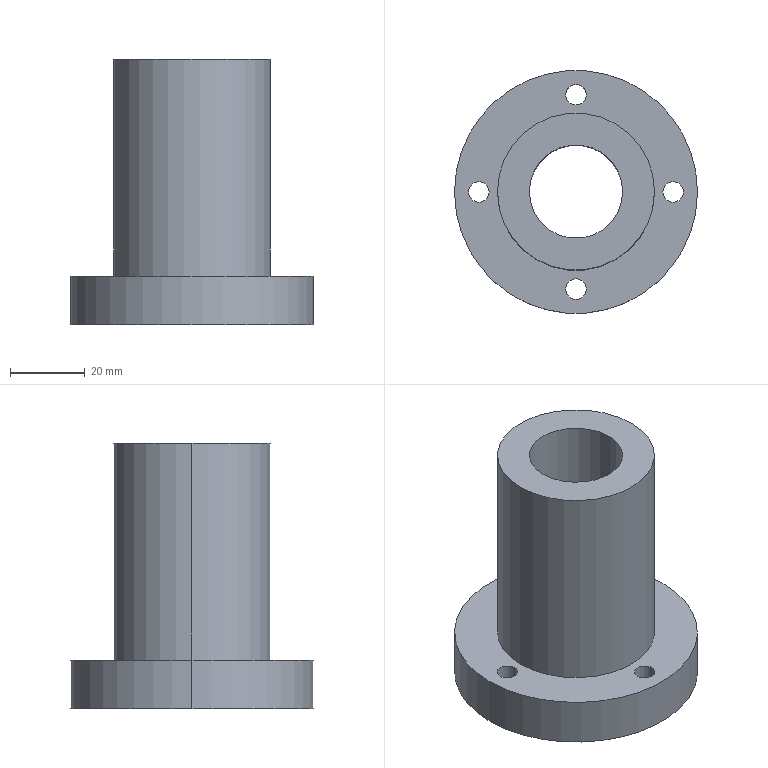Part | SolidWorks | features 3DProfileFeature 1, Extrusion 1, HoleWzd 1, ICE 1 | 1 solid | 29 faces | box 65 x 65 x 71 mm | volume 86157 mm3 | cylinder 22 | plane 7 | commonest cylinder face diameters 5.5 x8 10 x8 25 x2 42 x2 65 x2
STEP:
#1=CARTESIAN_POINT('',(5.,26.,5.7));
#2=VERTEX_POINT('',#1);
#3=CARTESIAN_POINT('',(-5.,26.,5.7));
#4=VERTEX_POINT('',#3);
#5=CARTESIAN_POINT('',(0.,26.,5.7));
#6=DIRECTION('',(0.,0.,-1.));
#7=DIRECTION('',(-1.,0.,0.));
#8=AXIS2_PLACEMENT_3D('',#5,#6,#7);
#9=CIRCLE('',#8,5.);
#10=EDGE_CURVE('',#2,#4,#9,.T.);
#11=ORIENTED_EDGE('',*,*,#10,.F.);
#12=CARTESIAN_POINT('',(5.,26.,0.));
#13=VERTEX_POINT('',#12);
#14=CARTESIAN_POINT('',(5.,26.,0.));
#15=DIRECTION('',(0.,0.,-1.));
#16=VECTOR('',#15,1000.);
#17=LINE('',#14,#16);
#18=EDGE_CURVE('',#2,#13,#17,.T.);
#19=ORIENTED_EDGE('',*,*,#18,.T.);
#20=CARTESIAN_POINT('',(-5.,26.,0.));
#21=VERTEX_POINT('',#20);
#22=CARTESIAN_POINT('',(0.,26.,0.));
#23=DIRECTION('',(0.,0.,-1.));
#24=DIRECTION('',(-1.,0.,0.));
#25=AXIS2_PLACEMENT_3D('',#22,#23,#24);
#26=CIRCLE('',#25,5.);
#27=EDGE_CURVE('',#13,#21,#26,.T.);
#28=ORIENTED_EDGE('',*,*,#27,.T.);
#29=CARTESIAN_POINT('',(-5.,26.,0.));
#30=DIRECTION('',(0.,0.,-1.));
#31=VECTOR('',#30,1000.);
#32=LINE('',#29,#31);
#33=EDGE_CURVE('',#4,#21,#32,.T.);
#34=ORIENTED_EDGE('',*,*,#33,.F.);
#35=EDGE_LOOP('',(#11,#19,#28,#34));
#36=FACE_OUTER_BOUND('',#35,.T.);
#37=CARTESIAN_POINT('',(0.,26.,0.));
#38=DIRECTION('',(0.,0.,-1.));
#39=DIRECTION('',(-1.,0.,0.));
#40=AXIS2_PLACEMENT_3D('',#37,#38,#39);
#41=CYLINDRICAL_SURFACE('',#40,5.);
#42=ADVANCED_FACE('',(#36),#41,.F.);
#43=CARTESIAN_POINT('',(2.75,26.,13.));
#44=VERTEX_POINT('',#43);
#45=CARTESIAN_POINT('',(-2.75,26.,13.));
#46=VERTEX_POINT('',#45);
#47=CARTESIAN_POINT('',(0.,26.,13.));
#48=DIRECTION('',(0.,0.,-1.));
#49=DIRECTION('',(-1.,0.,0.));
#50=AXIS2_PLACEMENT_3D('',#47,#48,#49);
#51=CIRCLE('',#50,2.75);
#52=EDGE_CURVE('',#44,#46,#51,.T.);
#53=ORIENTED_EDGE('',*,*,#52,.F.);
#54=CARTESIAN_POINT('',(2.75,26.,5.7));
#55=VERTEX_POINT('',#54);
#56=CARTESIAN_POINT('',(2.75,26.,0.));
#57=DIRECTION('',(0.,0.,-1.));
#58=VECTOR('',#57,1000.);
#59=LINE('',#56,#58);
#60=EDGE_CURVE('',#44,#55,#59,.T.);
#61=ORIENTED_EDGE('',*,*,#60,.T.);
#62=CARTESIAN_POINT('',(-2.75,26.,5.7));
#63=VERTEX_POINT('',#62);
#64=CARTESIAN_POINT('',(0.,26.,5.7));
#65=DIRECTION('',(0.,0.,-1.));
#66=DIRECTION('',(-1.,0.,0.));
#67=AXIS2_PLACEMENT_3D('',#64,#65,#66);
#68=CIRCLE('',#67,2.75);
#69=EDGE_CURVE('',#55,#63,#68,.T.);
#70=ORIENTED_EDGE('',*,*,#69,.T.);
#71=CARTESIAN_POINT('',(-2.75,26.,0.));
#72=DIRECTION('',(0.,0.,-1.));
#73=VECTOR('',#72,1000.);
#74=LINE('',#71,#73);
#75=EDGE_CURVE('',#46,#63,#74,.T.);
#76=ORIENTED_EDGE('',*,*,#75,.F.);
#77=EDGE_LOOP('',(#53,#61,#70,#76));
#78=FACE_OUTER_BOUND('',#77,.T.);
#79=CARTESIAN_POINT('',(0.,26.,0.));
#80=DIRECTION('',(0.,0.,-1.));
#81=DIRECTION('',(-1.,0.,0.));
#82=AXIS2_PLACEMENT_3D('',#79,#80,#81);
#83=CYLINDRICAL_SURFACE('',#82,2.75);
#84=ADVANCED_FACE('',(#78),#83,.F.);
#85=CARTESIAN_POINT('',(-21.,0.,5.7));
#86=VERTEX_POINT('',#85);
#87=CARTESIAN_POINT('',(-31.,0.,5.7));
#88=VERTEX_POINT('',#87);
#89=CARTESIAN_POINT('',(-26.,0.,5.7));
#90=DIRECTION('',(0.,0.,-1.));
#91=DIRECTION('',(-1.,0.,0.));
#92=AXIS2_PLACEMENT_3D('',#89,#90,#91);
#93=CIRCLE('',#92,5.);
#94=EDGE_CURVE('',#86,#88,#93,.T.);
#95=ORIENTED_EDGE('',*,*,#94,.F.);
#96=CARTESIAN_POINT('',(-21.,0.,0.));
#97=VERTEX_POINT('',#96);
#98=CARTESIAN_POINT('',(-21.,0.,0.));
#99=DIRECTION('',(0.,0.,-1.));
#100=VECTOR('',#99,1000.);
#101=LINE('',#98,#100);
#102=EDGE_CURVE('',#86,#97,#101,.T.);
#103=ORIENTED_EDGE('',*,*,#102,.T.);
#104=CARTESIAN_POINT('',(-31.,0.,0.));
#105=VERTEX_POINT('',#104);
#106=CARTESIAN_POINT('',(-26.,0.,0.));
#107=DIRECTION('',(0.,0.,-1.));
#108=DIRECTION('',(-1.,0.,0.));
#109=AXIS2_PLACEMENT_3D('',#106,#107,#108);
#110=CIRCLE('',#109,5.);
#111=EDGE_CURVE('',#97,#105,#110,.T.);
#112=ORIENTED_EDGE('',*,*,#111,.T.);
#113=CARTESIAN_POINT('',(-31.,0.,0.));
#114=DIRECTION('',(0.,0.,-1.));
#115=VECTOR('',#114,1000.);
#116=LINE('',#113,#115);
#117=EDGE_CURVE('',#88,#105,#116,.T.);
#118=ORIENTED_EDGE('',*,*,#117,.F.);
#119=EDGE_LOOP('',(#95,#103,#112,#118));
#120=FACE_OUTER_BOUND('',#119,.T.);
#121=CARTESIAN_POINT('',(-26.,0.,0.));
#122=DIRECTION('',(0.,0.,-1.));
#123=DIRECTION('',(-1.,0.,0.));
#124=AXIS2_PLACEMENT_3D('',#121,#122,#123);
#125=CYLINDRICAL_SURFACE('',#124,5.);
#126=ADVANCED_FACE('',(#120),#125,.F.);
#127=CARTESIAN_POINT('',(-23.25,0.,13.));
#128=VERTEX_POINT('',#127);
#129=CARTESIAN_POINT('',(-28.75,0.,13.));
#130=VERTEX_POINT('',#129);
#131=CARTESIAN_POINT('',(-26.,0.,13.));
#132=DIRECTION('',(0.,0.,-1.));
#133=DIRECTION('',(-1.,0.,0.));
#134=AXIS2_PLACEMENT_3D('',#131,#132,#133);
#135=CIRCLE('',#134,2.75);
#136=EDGE_CURVE('',#128,#130,#135,.T.);
#137=ORIENTED_EDGE('',*,*,#136,.F.);
#138=CARTESIAN_POINT('',(-23.25,0.,5.7));
#139=VERTEX_POINT('',#138);
#140=CARTESIAN_POINT('',(-23.25,0.,0.));
#141=DIRECTION('',(0.,0.,-1.));
#142=VECTOR('',#141,1000.);
#143=LINE('',#140,#142);
#144=EDGE_CURVE('',#128,#139,#143,.T.);
#145=ORIENTED_EDGE('',*,*,#144,.T.);
#146=CARTESIAN_POINT('',(-28.75,0.,5.7));
#147=VERTEX_POINT('',#146);
#148=CARTESIAN_POINT('',(-26.,0.,5.7));
#149=DIRECTION('',(0.,0.,-1.));
#150=DIRECTION('',(-1.,0.,0.));
#151=AXIS2_PLACEMENT_3D('',#148,#149,#150);
#152=CIRCLE('',#151,2.75);
#153=EDGE_CURVE('',#139,#147,#152,.T.);
#154=ORIENTED_EDGE('',*,*,#153,.T.);
#155=CARTESIAN_POINT('',(-28.75,0.,0.));
#156=DIRECTION('',(0.,0.,-1.));
#157=VECTOR('',#156,1000.);
#158=LINE('',#155,#157);
#159=EDGE_CURVE('',#130,#147,#158,.T.);
#160=ORIENTED_EDGE('',*,*,#159,.F.);
#161=EDGE_LOOP('',(#137,#145,#154,#160));
#162=FACE_OUTER_BOUND('',#161,.T.);
#163=CARTESIAN_POINT('',(-26.,0.,0.));
#164=DIRECTION('',(0.,0.,-1.));
#165=DIRECTION('',(-1.,0.,0.));
#166=AXIS2_PLACEMENT_3D('',#163,#164,#165);
#167=CYLINDRICAL_SURFACE('',#166,2.75);
#168=ADVANCED_FACE('',(#162),#167,.F.);
#169=CARTESIAN_POINT('',(5.,-26.,5.7));
#170=VERTEX_POINT('',#169);
#171=CARTESIAN_POINT('',(-5.,-26.,5.7));
#172=VERTEX_POINT('',#171);
#173=CARTESIAN_POINT('',(0.,-26.,5.7));
#174=DIRECTION('',(0.,0.,-1.));
#175=DIRECTION('',(-1.,0.,0.));
#176=AXIS2_PLACEMENT_3D('',#173,#174,#175);
#177=CIRCLE('',#176,5.);
#178=EDGE_CURVE('',#170,#172,#177,.T.);
#179=ORIENTED_EDGE('',*,*,#178,.F.);
#180=CARTESIAN_POINT('',(5.,-26.,0.));
#181=VERTEX_POINT('',#180);
#182=CARTESIAN_POINT('',(5.,-26.,0.));
#183=DIRECTION('',(0.,0.,-1.));
#184=VECTOR('',#183,1000.);
#185=LINE('',#182,#184);
#186=EDGE_CURVE('',#170,#181,#185,.T.);
#187=ORIENTED_EDGE('',*,*,#186,.T.);
#188=CARTESIAN_POINT('',(-5.,-26.,0.));
#189=VERTEX_POINT('',#188);
#190=CARTESIAN_POINT('',(0.,-26.,0.));
#191=DIRECTION('',(0.,0.,-1.));
#192=DIRECTION('',(-1.,0.,0.));
#193=AXIS2_PLACEMENT_3D('',#190,#191,#192);
#194=CIRCLE('',#193,5.);
#195=EDGE_CURVE('',#181,#189,#194,.T.);
#196=ORIENTED_EDGE('',*,*,#195,.T.);
#197=CARTESIAN_POINT('',(-5.,-26.,0.));
#198=DIRECTION('',(0.,0.,-1.));
#199=VECTOR('',#198,1000.);
#200=LINE('',#197,#199);
#201=EDGE_CURVE('',#172,#189,#200,.T.);
#202=ORIENTED_EDGE('',*,*,#201,.F.);
#203=EDGE_LOOP('',(#179,#187,#196,#202));
#204=FACE_OUTER_BOUND('',#203,.T.);
#205=CARTESIAN_POINT('',(0.,-26.,0.));
#206=DIRECTION('',(0.,0.,-1.));
#207=DIRECTION('',(-1.,0.,0.));
#208=AXIS2_PLACEMENT_3D('',#205,#206,#207);
#209=CYLINDRICAL_SURFACE('',#208,5.);
#210=ADVANCED_FACE('',(#204),#209,.F.);
#211=CARTESIAN_POINT('',(2.75,-26.,13.));
#212=VERTEX_POINT('',#211);
#213=CARTESIAN_POINT('',(-2.75,-26.,13.));
#214=VERTEX_POINT('',#213);
#215=CARTESIAN_POINT('',(0.,-26.,13.));
#216=DIRECTION('',(0.,0.,-1.));
#217=DIRECTION('',(-1.,0.,0.));
#218=AXIS2_PLACEMENT_3D('',#215,#216,#217);
#219=CIRCLE('',#218,2.75);
#220=EDGE_CURVE('',#212,#214,#219,.T.);
#221=ORIENTED_EDGE('',*,*,#220,.F.);
#222=CARTESIAN_POINT('',(2.75,-26.,5.7));
#223=VERTEX_POINT('',#222);
#224=CARTESIAN_POINT('',(2.75,-26.,0.));
#225=DIRECTION('',(0.,0.,-1.));
#226=VECTOR('',#225,1000.);
#227=LINE('',#224,#226);
#228=EDGE_CURVE('',#212,#223,#227,.T.);
#229=ORIENTED_EDGE('',*,*,#228,.T.);
#230=CARTESIAN_POINT('',(-2.75,-26.,5.7));
#231=VERTEX_POINT('',#230);
#232=CARTESIAN_POINT('',(0.,-26.,5.7));
#233=DIRECTION('',(0.,0.,-1.));
#234=DIRECTION('',(-1.,0.,0.));
#235=AXIS2_PLACEMENT_3D('',#232,#233,#234);
#236=CIRCLE('',#235,2.75);
#237=EDGE_CURVE('',#223,#231,#236,.T.);
#238=ORIENTED_EDGE('',*,*,#237,.T.);
#239=CARTESIAN_POINT('',(-2.75,-26.,0.));
#240=DIRECTION('',(0.,0.,-1.));
#241=VECTOR('',#240,1000.);
#242=LINE('',#239,#241);
#243=EDGE_CURVE('',#214,#231,#242,.T.);
#244=ORIENTED_EDGE('',*,*,#243,.F.);
#245=EDGE_LOOP('',(#221,#229,#238,#244));
#246=FACE_OUTER_BOUND('',#245,.T.);
#247=CARTESIAN_POINT('',(0.,-26.,0.));
#248=DIRECTION('',(0.,0.,-1.));
#249=DIRECTION('',(-1.,0.,0.));
#250=AXIS2_PLACEMENT_3D('',#247,#248,#249);
#251=CYLINDRICAL_SURFACE('',#250,2.75);
#252=ADVANCED_FACE('',(#246),#251,.F.);
#253=CARTESIAN_POINT('',(31.,0.,5.7));
#254=VERTEX_POINT('',#253);
#255=CARTESIAN_POINT('',(21.,0.,5.7));
#256=VERTEX_POINT('',#255);
#257=CARTESIAN_POINT('',(26.,0.,5.7));
#258=DIRECTION('',(0.,0.,-1.));
#259=DIRECTION('',(-1.,0.,0.));
#260=AXIS2_PLACEMENT_3D('',#257,#258,#259);
#261=CIRCLE('',#260,5.);
#262=EDGE_CURVE('',#254,#256,#261,.T.);
#263=ORIENTED_EDGE('',*,*,#262,.F.);
#264=CARTESIAN_POINT('',(31.,0.,0.));
#265=VERTEX_POINT('',#264);
#266=CARTESIAN_POINT('',(31.,0.,0.));
#267=DIRECTION('',(0.,0.,-1.));
#268=VECTOR('',#267,1000.);
#269=LINE('',#266,#268);
#270=EDGE_CURVE('',#254,#265,#269,.T.);
#271=ORIENTED_EDGE('',*,*,#270,.T.);
#272=CARTESIAN_POINT('',(21.,0.,0.));
#273=VERTEX_POINT('',#272);
#274=CARTESIAN_POINT('',(26.,0.,0.));
#275=DIRECTION('',(0.,0.,-1.));
#276=DIRECTION('',(-1.,0.,0.));
#277=AXIS2_PLACEMENT_3D('',#274,#275,#276);
#278=CIRCLE('',#277,5.);
#279=EDGE_CURVE('',#265,#273,#278,.T.);
#280=ORIENTED_EDGE('',*,*,#279,.T.);
#281=CARTESIAN_POINT('',(21.,0.,0.));
#282=DIRECTION('',(0.,0.,-1.));
#283=VECTOR('',#282,1000.);
#284=LINE('',#281,#283);
#285=EDGE_CURVE('',#256,#273,#284,.T.);
#286=ORIENTED_EDGE('',*,*,#285,.F.);
#287=EDGE_LOOP('',(#263,#271,#280,#286));
#288=FACE_OUTER_BOUND('',#287,.T.);
#289=CARTESIAN_POINT('',(26.,0.,0.));
#290=DIRECTION('',(0.,0.,-1.));
#291=DIRECTION('',(-1.,0.,0.));
#292=AXIS2_PLACEMENT_3D('',#289,#290,#291);
#293=CYLINDRICAL_SURFACE('',#292,5.);
#294=ADVANCED_FACE('',(#288),#293,.F.);
#295=CARTESIAN_POINT('',(28.75,0.,13.));
#296=VERTEX_POINT('',#295);
#297=CARTESIAN_POINT('',(23.25,0.,13.));
#298=VERTEX_POINT('',#297);
#299=CARTESIAN_POINT('',(26.,0.,13.));
#300=DIRECTION('',(0.,0.,-1.));
#301=DIRECTION('',(-1.,0.,0.));
#302=AXIS2_PLACEMENT_3D('',#299,#300,#301);
#303=CIRCLE('',#302,2.75);
#304=EDGE_CURVE('',#296,#298,#303,.T.);
#305=ORIENTED_EDGE('',*,*,#304,.F.);
#306=CARTESIAN_POINT('',(28.75,0.,5.7));
#307=VERTEX_POINT('',#306);
#308=CARTESIAN_POINT('',(28.75,0.,0.));
#309=DIRECTION('',(0.,0.,-1.));
#310=VECTOR('',#309,1000.);
#311=LINE('',#308,#310);
#312=EDGE_CURVE('',#296,#307,#311,.T.);
#313=ORIENTED_EDGE('',*,*,#312,.T.);
#314=CARTESIAN_POINT('',(23.25,0.,5.7));
#315=VERTEX_POINT('',#314);
#316=CARTESIAN_POINT('',(26.,0.,5.7));
#317=DIRECTION('',(0.,0.,-1.));
#318=DIRECTION('',(-1.,0.,0.));
#319=AXIS2_PLACEMENT_3D('',#316,#317,#318);
#320=CIRCLE('',#319,2.75);
#321=EDGE_CURVE('',#307,#315,#320,.T.);
#322=ORIENTED_EDGE('',*,*,#321,.T.);
#323=CARTESIAN_POINT('',(23.25,0.,0.));
#324=DIRECTION('',(0.,0.,-1.));
#325=VECTOR('',#324,1000.);
#326=LINE('',#323,#325);
#327=EDGE_CURVE('',#298,#315,#326,.T.);
#328=ORIENTED_EDGE('',*,*,#327,.F.);
#329=EDGE_LOOP('',(#305,#313,#322,#328));
#330=FACE_OUTER_BOUND('',#329,.T.);
#331=CARTESIAN_POINT('',(26.,0.,0.));
#332=DIRECTION('',(0.,0.,-1.));
#333=DIRECTION('',(-1.,0.,0.));
#334=AXIS2_PLACEMENT_3D('',#331,#332,#333);
#335=CYLINDRICAL_SURFACE('',#334,2.75);
#336=ADVANCED_FACE('',(#330),#335,.F.);
#337=CARTESIAN_POINT('',(-32.5,0.,13.));
#338=VERTEX_POINT('',#337);
#339=CARTESIAN_POINT('',(32.5,0.,13.));
#340=VERTEX_POINT('',#339);
#341=CARTESIAN_POINT('',(0.,0.,13.));
#342=DIRECTION('',(0.,0.,-1.));
#343=DIRECTION('',(-1.,0.,0.));
#344=AXIS2_PLACEMENT_3D('',#341,#342,#343);
#345=CIRCLE('',#344,32.5);
#346=EDGE_CURVE('',#338,#340,#345,.T.);
#347=ORIENTED_EDGE('',*,*,#346,.T.);
#348=CARTESIAN_POINT('',(32.5,0.,0.));
#349=VERTEX_POINT('',#348);
#350=CARTESIAN_POINT('',(32.5,0.,13.));
#351=DIRECTION('',(0.,0.,-1.));
#352=VECTOR('',#351,1000.);
#353=LINE('',#350,#352);
#354=EDGE_CURVE('',#340,#349,#353,.T.);
#355=ORIENTED_EDGE('',*,*,#354,.T.);
#356=CARTESIAN_POINT('',(-32.5,0.,0.));
#357=VERTEX_POINT('',#356);
#358=CARTESIAN_POINT('',(0.,0.,0.));
#359=DIRECTION('',(0.,0.,-1.));
#360=DIRECTION('',(-1.,0.,0.));
#361=AXIS2_PLACEMENT_3D('',#358,#359,#360);
#362=CIRCLE('',#361,32.5);
#363=EDGE_CURVE('',#357,#349,#362,.T.);
#364=ORIENTED_EDGE('',*,*,#363,.F.);
#365=CARTESIAN_POINT('',(-32.5,0.,13.));
#366=DIRECTION('',(0.,0.,-1.));
#367=VECTOR('',#366,1000.);
#368=LINE('',#365,#367);
#369=EDGE_CURVE('',#338,#357,#368,.T.);
#370=ORIENTED_EDGE('',*,*,#369,.F.);
#371=EDGE_LOOP('',(#347,#355,#364,#370));
#372=FACE_OUTER_BOUND('',#371,.T.);
#373=CARTESIAN_POINT('',(0.,0.,13.));
#374=DIRECTION('',(0.,0.,-1.));
#375=DIRECTION('',(-1.,0.,0.));
#376=AXIS2_PLACEMENT_3D('',#373,#374,#375);
#377=CYLINDRICAL_SURFACE('',#376,32.5);
#378=ADVANCED_FACE('',(#372),#377,.T.);
#379=CARTESIAN_POINT('',(-12.5,0.,71.));
#380=VERTEX_POINT('',#379);
#381=CARTESIAN_POINT('',(12.5,0.,71.));
#382=VERTEX_POINT('',#381);
#383=CARTESIAN_POINT('',(0.,0.,71.));
#384=DIRECTION('',(0.,0.,1.));
#385=DIRECTION('',(1.,0.,0.));
#386=AXIS2_PLACEMENT_3D('',#383,#384,#385);
#387=CIRCLE('',#386,12.5);
#388=EDGE_CURVE('',#380,#382,#387,.T.);
#389=ORIENTED_EDGE('',*,*,#388,.T.);
#390=CARTESIAN_POINT('',(12.5,0.,0.));
#391=VERTEX_POINT('',#390);
#392=CARTESIAN_POINT('',(12.5,0.,71.));
#393=DIRECTION('',(0.,0.,-1.));
#394=VECTOR('',#393,1000.);
#395=LINE('',#392,#394);
#396=EDGE_CURVE('',#382,#391,#395,.T.);
#397=ORIENTED_EDGE('',*,*,#396,.T.);
#398=CARTESIAN_POINT('',(-12.5,0.,0.));
#399=VERTEX_POINT('',#398);
#400=CARTESIAN_POINT('',(0.,0.,0.));
#401=DIRECTION('',(0.,0.,1.));
#402=DIRECTION('',(1.,0.,0.));
#403=AXIS2_PLACEMENT_3D('',#400,#401,#402);
#404=CIRCLE('',#403,12.5);
#405=EDGE_CURVE('',#399,#391,#404,.T.);
#406=ORIENTED_EDGE('',*,*,#405,.F.);
#407=CARTESIAN_POINT('',(-12.5,0.,71.));
#408=DIRECTION('',(0.,0.,-1.));
#409=VECTOR('',#408,1000.);
#410=LINE('',#407,#409);
#411=EDGE_CURVE('',#380,#399,#410,.T.);
#412=ORIENTED_EDGE('',*,*,#411,.F.);
#413=EDGE_LOOP('',(#389,#397,#406,#412));
#414=FACE_OUTER_BOUND('',#413,.T.);
#415=CARTESIAN_POINT('',(0.,0.,71.));
#416=DIRECTION('',(0.,0.,-1.));
#417=DIRECTION('',(-1.,0.,0.));
#418=AXIS2_PLACEMENT_3D('',#415,#416,#417);
#419=CYLINDRICAL_SURFACE('',#418,12.5);
#420=ADVANCED_FACE('',(#414),#419,.F.);
#421=CARTESIAN_POINT('',(21.,0.,71.));
#422=VERTEX_POINT('',#421);
#423=CARTESIAN_POINT('',(-21.,0.,71.));
#424=VERTEX_POINT('',#423);
#425=CARTESIAN_POINT('',(0.,0.,71.));
#426=DIRECTION('',(0.,0.,1.));
#427=DIRECTION('',(1.,0.,0.));
#428=AXIS2_PLACEMENT_3D('',#425,#426,#427);
#429=CIRCLE('',#428,21.);
#430=EDGE_CURVE('',#422,#424,#429,.T.);
#431=ORIENTED_EDGE('',*,*,#430,.F.);
#432=CARTESIAN_POINT('',(21.,0.,13.));
#433=VERTEX_POINT('',#432);
#434=CARTESIAN_POINT('',(21.,0.,71.));
#435=DIRECTION('',(0.,0.,-1.));
#436=VECTOR('',#435,1000.);
#437=LINE('',#434,#436);
#438=EDGE_CURVE('',#422,#433,#437,.T.);
#439=ORIENTED_EDGE('',*,*,#438,.T.);
#440=CARTESIAN_POINT('',(-21.,0.,13.));
#441=VERTEX_POINT('',#440);
#442=CARTESIAN_POINT('',(0.,0.,13.));
#443=DIRECTION('',(0.,0.,-1.));
#444=DIRECTION('',(-1.,0.,0.));
#445=AXIS2_PLACEMENT_3D('',#442,#443,#444);
#446=CIRCLE('',#445,21.);
#447=EDGE_CURVE('',#441,#433,#446,.T.);
#448=ORIENTED_EDGE('',*,*,#447,.F.);
#449=CARTESIAN_POINT('',(-21.,0.,71.));
#450=DIRECTION('',(0.,0.,-1.));
#451=VECTOR('',#450,1000.);
#452=LINE('',#449,#451);
#453=EDGE_CURVE('',#424,#441,#452,.T.);
#454=ORIENTED_EDGE('',*,*,#453,.F.);
#455=EDGE_LOOP('',(#431,#439,#448,#454));
#456=FACE_OUTER_BOUND('',#455,.T.);
#457=CARTESIAN_POINT('',(0.,0.,71.));
#458=DIRECTION('',(0.,0.,-1.));
#459=DIRECTION('',(-1.,0.,0.));
#460=AXIS2_PLACEMENT_3D('',#457,#458,#459);
#461=CYLINDRICAL_SURFACE('',#460,21.);
#462=ADVANCED_FACE('',(#456),#461,.T.);
#463=CARTESIAN_POINT('',(26.,0.,0.));
#464=DIRECTION('',(0.,0.,-1.));
#465=DIRECTION('',(-1.,0.,0.));
#466=AXIS2_PLACEMENT_3D('',#463,#464,#465);
#467=CIRCLE('',#466,5.);
#468=EDGE_CURVE('',#273,#265,#467,.T.);
#469=ORIENTED_EDGE('',*,*,#468,.F.);
#470=ORIENTED_EDGE('',*,*,#279,.F.);
#471=EDGE_LOOP('',(#469,#470));
#472=FACE_BOUND('',#471,.T.);
#473=ORIENTED_EDGE('',*,*,#405,.T.);
#474=CARTESIAN_POINT('',(0.,0.,0.));
#475=DIRECTION('',(0.,0.,1.));
#476=DIRECTION('',(1.,0.,0.));
#477=AXIS2_PLACEMENT_3D('',#474,#475,#476);
#478=CIRCLE('',#477,12.5);
#479=EDGE_CURVE('',#391,#399,#478,.T.);
#480=ORIENTED_EDGE('',*,*,#479,.T.);
#481=EDGE_LOOP('',(#473,#480));
#482=FACE_BOUND('',#481,.T.);
#483=ORIENTED_EDGE('',*,*,#363,.T.);
#484=CARTESIAN_POINT('',(0.,0.,0.));
#485=DIRECTION('',(0.,0.,-1.));
#486=DIRECTION('',(-1.,0.,0.));
#487=AXIS2_PLACEMENT_3D('',#484,#485,#486);
#488=CIRCLE('',#487,32.5);
#489=EDGE_CURVE('',#349,#357,#488,.T.);
#490=ORIENTED_EDGE('',*,*,#489,.T.);
#491=EDGE_LOOP('',(#483,#490));
#492=FACE_OUTER_BOUND('',#491,.T.);
#493=CARTESIAN_POINT('',(0.,-26.,0.));
#494=DIRECTION('',(0.,0.,-1.));
#495=DIRECTION('',(-1.,0.,0.));
#496=AXIS2_PLACEMENT_3D('',#493,#494,#495);
#497=CIRCLE('',#496,5.);
#498=EDGE_CURVE('',#189,#181,#497,.T.);
#499=ORIENTED_EDGE('',*,*,#498,.F.);
#500=ORIENTED_EDGE('',*,*,#195,.F.);
#501=EDGE_LOOP('',(#499,#500));
#502=FACE_BOUND('',#501,.T.);
#503=CARTESIAN_POINT('',(-26.,0.,0.));
#504=DIRECTION('',(0.,0.,-1.));
#505=DIRECTION('',(-1.,0.,0.));
#506=AXIS2_PLACEMENT_3D('',#503,#504,#505);
#507=CIRCLE('',#506,5.);
#508=EDGE_CURVE('',#105,#97,#507,.T.);
#509=ORIENTED_EDGE('',*,*,#508,.F.);
#510=ORIENTED_EDGE('',*,*,#111,.F.);
#511=EDGE_LOOP('',(#509,#510));
#512=FACE_BOUND('',#511,.T.);
#513=CARTESIAN_POINT('',(0.,26.,0.));
#514=DIRECTION('',(0.,0.,-1.));
#515=DIRECTION('',(-1.,0.,0.));
#516=AXIS2_PLACEMENT_3D('',#513,#514,#515);
#517=CIRCLE('',#516,5.);
#518=EDGE_CURVE('',#21,#13,#517,.T.);
#519=ORIENTED_EDGE('',*,*,#518,.F.);
#520=ORIENTED_EDGE('',*,*,#27,.F.);
#521=EDGE_LOOP('',(#519,#520));
#522=FACE_BOUND('',#521,.T.);
#523=CARTESIAN_POINT('',(0.,0.,0.));
#524=DIRECTION('',(0.,0.,1.));
#525=DIRECTION('',(1.,0.,0.));
#526=AXIS2_PLACEMENT_3D('',#523,#524,#525);
#527=PLANE('',#526);
#528=ADVANCED_FACE('',(#472,#482,#492,#502,#512,#522),#527,.F.);
#529=ORIENTED_EDGE('',*,*,#438,.F.);
#530=CARTESIAN_POINT('',(0.,0.,71.));
#531=DIRECTION('',(0.,0.,1.));
#532=DIRECTION('',(1.,0.,0.));
#533=AXIS2_PLACEMENT_3D('',#530,#531,#532);
#534=CIRCLE('',#533,21.);
#535=EDGE_CURVE('',#424,#422,#534,.T.);
#536=ORIENTED_EDGE('',*,*,#535,.F.);
#537=ORIENTED_EDGE('',*,*,#453,.T.);
#538=CARTESIAN_POINT('',(0.,0.,13.));
#539=DIRECTION('',(0.,0.,-1.));
#540=DIRECTION('',(-1.,0.,0.));
#541=AXIS2_PLACEMENT_3D('',#538,#539,#540);
#542=CIRCLE('',#541,21.);
#543=EDGE_CURVE('',#433,#441,#542,.T.);
#544=ORIENTED_EDGE('',*,*,#543,.F.);
#545=EDGE_LOOP('',(#529,#536,#537,#544));
#546=FACE_OUTER_BOUND('',#545,.T.);
#547=CARTESIAN_POINT('',(0.,0.,71.));
#548=DIRECTION('',(0.,0.,-1.));
#549=DIRECTION('',(-1.,0.,0.));
#550=AXIS2_PLACEMENT_3D('',#547,#548,#549);
#551=CYLINDRICAL_SURFACE('',#550,21.);
#552=ADVANCED_FACE('',(#546),#551,.T.);
#553=ORIENTED_EDGE('',*,*,#535,.T.);
#554=ORIENTED_EDGE('',*,*,#430,.T.);
#555=EDGE_LOOP('',(#553,#554));
#556=FACE_OUTER_BOUND('',#555,.T.);
#557=ORIENTED_EDGE('',*,*,#388,.F.);
#558=CARTESIAN_POINT('',(0.,0.,71.));
#559=DIRECTION('',(0.,0.,1.));
#560=DIRECTION('',(1.,0.,0.));
#561=AXIS2_PLACEMENT_3D('',#558,#559,#560);
#562=CIRCLE('',#561,12.5);
#563=EDGE_CURVE('',#382,#380,#562,.T.);
#564=ORIENTED_EDGE('',*,*,#563,.F.);
#565=EDGE_LOOP('',(#557,#564));
#566=FACE_BOUND('',#565,.T.);
#567=CARTESIAN_POINT('',(0.,0.,71.));
#568=DIRECTION('',(0.,0.,1.));
#569=DIRECTION('',(1.,0.,0.));
#570=AXIS2_PLACEMENT_3D('',#567,#568,#569);
#571=PLANE('',#570);
#572=ADVANCED_FACE('',(#556,#566),#571,.T.);
#573=ORIENTED_EDGE('',*,*,#396,.F.);
#574=ORIENTED_EDGE('',*,*,#563,.T.);
#575=ORIENTED_EDGE('',*,*,#411,.T.);
#576=ORIENTED_EDGE('',*,*,#479,.F.);
#577=EDGE_LOOP('',(#573,#574,#575,#576));
#578=FACE_OUTER_BOUND('',#577,.T.);
#579=CARTESIAN_POINT('',(0.,0.,71.));
#580=DIRECTION('',(0.,0.,-1.));
#581=DIRECTION('',(-1.,0.,0.));
#582=AXIS2_PLACEMENT_3D('',#579,#580,#581);
#583=CYLINDRICAL_SURFACE('',#582,12.5);
#584=ADVANCED_FACE('',(#578),#583,.F.);
#585=CARTESIAN_POINT('',(0.,26.,13.));
#586=DIRECTION('',(0.,0.,-1.));
#587=DIRECTION('',(-1.,0.,0.));
#588=AXIS2_PLACEMENT_3D('',#585,#586,#587);
#589=CIRCLE('',#588,2.75);
#590=EDGE_CURVE('',#46,#44,#589,.T.);
#591=ORIENTED_EDGE('',*,*,#590,.T.);
#592=ORIENTED_EDGE('',*,*,#52,.T.);
#593=EDGE_LOOP('',(#591,#592));
#594=FACE_BOUND('',#593,.T.);
#595=CARTESIAN_POINT('',(-26.,0.,13.));
#596=DIRECTION('',(0.,0.,-1.));
#597=DIRECTION('',(-1.,0.,0.));
#598=AXIS2_PLACEMENT_3D('',#595,#596,#597);
#599=CIRCLE('',#598,2.75);
#600=EDGE_CURVE('',#130,#128,#599,.T.);
#601=ORIENTED_EDGE('',*,*,#600,.T.);
#602=ORIENTED_EDGE('',*,*,#136,.T.);
#603=EDGE_LOOP('',(#601,#602));
#604=FACE_BOUND('',#603,.T.);
#605=CARTESIAN_POINT('',(0.,-26.,13.));
#606=DIRECTION('',(0.,0.,-1.));
#607=DIRECTION('',(-1.,0.,0.));
#608=AXIS2_PLACEMENT_3D('',#605,#606,#607);
#609=CIRCLE('',#608,2.75);
#610=EDGE_CURVE('',#214,#212,#609,.T.);
#611=ORIENTED_EDGE('',*,*,#610,.T.);
#612=ORIENTED_EDGE('',*,*,#220,.T.);
#613=EDGE_LOOP('',(#611,#612));
#614=FACE_BOUND('',#613,.T.);
#615=CARTESIAN_POINT('',(26.,0.,13.));
#616=DIRECTION('',(0.,0.,-1.));
#617=DIRECTION('',(-1.,0.,0.));
#618=AXIS2_PLACEMENT_3D('',#615,#616,#617);
#619=CIRCLE('',#618,2.75);
#620=EDGE_CURVE('',#298,#296,#619,.T.);
#621=ORIENTED_EDGE('',*,*,#620,.T.);
#622=ORIENTED_EDGE('',*,*,#304,.T.);
#623=EDGE_LOOP('',(#621,#622));
#624=FACE_BOUND('',#623,.T.);
#625=ORIENTED_EDGE('',*,*,#346,.F.);
#626=CARTESIAN_POINT('',(0.,0.,13.));
#627=DIRECTION('',(0.,0.,-1.));
#628=DIRECTION('',(-1.,0.,0.));
#629=AXIS2_PLACEMENT_3D('',#626,#627,#628);
#630=CIRCLE('',#629,32.5);
#631=EDGE_CURVE('',#340,#338,#630,.T.);
#632=ORIENTED_EDGE('',*,*,#631,.F.);
#633=EDGE_LOOP('',(#625,#632));
#634=FACE_OUTER_BOUND('',#633,.T.);
#635=ORIENTED_EDGE('',*,*,#447,.T.);
#636=ORIENTED_EDGE('',*,*,#543,.T.);
#637=EDGE_LOOP('',(#635,#636));
#638=FACE_BOUND('',#637,.T.);
#639=CARTESIAN_POINT('',(0.,0.,13.));
#640=DIRECTION('',(0.,0.,-1.));
#641=DIRECTION('',(-1.,0.,0.));
#642=AXIS2_PLACEMENT_3D('',#639,#640,#641);
#643=PLANE('',#642);
#644=ADVANCED_FACE('',(#594,#604,#614,#624,#634,#638),#643,.F.);
#645=ORIENTED_EDGE('',*,*,#354,.F.);
#646=ORIENTED_EDGE('',*,*,#631,.T.);
#647=ORIENTED_EDGE('',*,*,#369,.T.);
#648=ORIENTED_EDGE('',*,*,#489,.F.);
#649=EDGE_LOOP('',(#645,#646,#647,#648));
#650=FACE_OUTER_BOUND('',#649,.T.);
#651=CARTESIAN_POINT('',(0.,0.,13.));
#652=DIRECTION('',(0.,0.,-1.));
#653=DIRECTION('',(-1.,0.,0.));
#654=AXIS2_PLACEMENT_3D('',#651,#652,#653);
#655=CYLINDRICAL_SURFACE('',#654,32.5);
#656=ADVANCED_FACE('',(#650),#655,.T.);
#657=ORIENTED_EDGE('',*,*,#312,.F.);
#658=ORIENTED_EDGE('',*,*,#620,.F.);
#659=ORIENTED_EDGE('',*,*,#327,.T.);
#660=CARTESIAN_POINT('',(26.,0.,5.7));
#661=DIRECTION('',(0.,0.,-1.));
#662=DIRECTION('',(-1.,0.,0.));
#663=AXIS2_PLACEMENT_3D('',#660,#661,#662);
#664=CIRCLE('',#663,2.75);
#665=EDGE_CURVE('',#315,#307,#664,.T.);
#666=ORIENTED_EDGE('',*,*,#665,.T.);
#667=EDGE_LOOP('',(#657,#658,#659,#666));
#668=FACE_OUTER_BOUND('',#667,.T.);
#669=CARTESIAN_POINT('',(26.,0.,0.));
#670=DIRECTION('',(0.,0.,-1.));
#671=DIRECTION('',(-1.,0.,0.));
#672=AXIS2_PLACEMENT_3D('',#669,#670,#671);
#673=CYLINDRICAL_SURFACE('',#672,2.75);
#674=ADVANCED_FACE('',(#668),#673,.F.);
#675=ORIENTED_EDGE('',*,*,#665,.F.);
#676=ORIENTED_EDGE('',*,*,#321,.F.);
#677=EDGE_LOOP('',(#675,#676));
#678=FACE_BOUND('',#677,.T.);
#679=CARTESIAN_POINT('',(26.,0.,5.7));
#680=DIRECTION('',(0.,0.,-1.));
#681=DIRECTION('',(-1.,0.,0.));
#682=AXIS2_PLACEMENT_3D('',#679,#680,#681);
#683=CIRCLE('',#682,5.);
#684=EDGE_CURVE('',#256,#254,#683,.T.);
#685=ORIENTED_EDGE('',*,*,#684,.T.);
#686=ORIENTED_EDGE('',*,*,#262,.T.);
#687=EDGE_LOOP('',(#685,#686));
#688=FACE_OUTER_BOUND('',#687,.T.);
#689=CARTESIAN_POINT('',(28.75,0.,5.7));
#690=DIRECTION('',(0.,0.,1.));
#691=DIRECTION('',(1.,0.,0.));
#692=AXIS2_PLACEMENT_3D('',#689,#690,#691);
#693=PLANE('',#692);
#694=ADVANCED_FACE('',(#678,#688),#693,.F.);
#695=ORIENTED_EDGE('',*,*,#270,.F.);
#696=ORIENTED_EDGE('',*,*,#684,.F.);
#697=ORIENTED_EDGE('',*,*,#285,.T.);
#698=ORIENTED_EDGE('',*,*,#468,.T.);
#699=EDGE_LOOP('',(#695,#696,#697,#698));
#700=FACE_OUTER_BOUND('',#699,.T.);
#701=CARTESIAN_POINT('',(26.,0.,0.));
#702=DIRECTION('',(0.,0.,-1.));
#703=DIRECTION('',(-1.,0.,0.));
#704=AXIS2_PLACEMENT_3D('',#701,#702,#703);
#705=CYLINDRICAL_SURFACE('',#704,5.);
#706=ADVANCED_FACE('',(#700),#705,.F.);
#707=ORIENTED_EDGE('',*,*,#228,.F.);
#708=ORIENTED_EDGE('',*,*,#610,.F.);
#709=ORIENTED_EDGE('',*,*,#243,.T.);
#710=CARTESIAN_POINT('',(0.,-26.,5.7));
#711=DIRECTION('',(0.,0.,-1.));
#712=DIRECTION('',(-1.,0.,0.));
#713=AXIS2_PLACEMENT_3D('',#710,#711,#712);
#714=CIRCLE('',#713,2.75);
#715=EDGE_CURVE('',#231,#223,#714,.T.);
#716=ORIENTED_EDGE('',*,*,#715,.T.);
#717=EDGE_LOOP('',(#707,#708,#709,#716));
#718=FACE_OUTER_BOUND('',#717,.T.);
#719=CARTESIAN_POINT('',(0.,-26.,0.));
#720=DIRECTION('',(0.,0.,-1.));
#721=DIRECTION('',(-1.,0.,0.));
#722=AXIS2_PLACEMENT_3D('',#719,#720,#721);
#723=CYLINDRICAL_SURFACE('',#722,2.75);
#724=ADVANCED_FACE('',(#718),#723,.F.);
#725=ORIENTED_EDGE('',*,*,#715,.F.);
#726=ORIENTED_EDGE('',*,*,#237,.F.);
#727=EDGE_LOOP('',(#725,#726));
#728=FACE_BOUND('',#727,.T.);
#729=CARTESIAN_POINT('',(0.,-26.,5.7));
#730=DIRECTION('',(0.,0.,-1.));
#731=DIRECTION('',(-1.,0.,0.));
#732=AXIS2_PLACEMENT_3D('',#729,#730,#731);
#733=CIRCLE('',#732,5.);
#734=EDGE_CURVE('',#172,#170,#733,.T.);
#735=ORIENTED_EDGE('',*,*,#734,.T.);
#736=ORIENTED_EDGE('',*,*,#178,.T.);
#737=EDGE_LOOP('',(#735,#736));
#738=FACE_OUTER_BOUND('',#737,.T.);
#739=CARTESIAN_POINT('',(2.75,-26.,5.7));
#740=DIRECTION('',(0.,0.,1.));
#741=DIRECTION('',(1.,0.,0.));
#742=AXIS2_PLACEMENT_3D('',#739,#740,#741);
#743=PLANE('',#742);
#744=ADVANCED_FACE('',(#728,#738),#743,.F.);
#745=ORIENTED_EDGE('',*,*,#186,.F.);
#746=ORIENTED_EDGE('',*,*,#734,.F.);
#747=ORIENTED_EDGE('',*,*,#201,.T.);
#748=ORIENTED_EDGE('',*,*,#498,.T.);
#749=EDGE_LOOP('',(#745,#746,#747,#748));
#750=FACE_OUTER_BOUND('',#749,.T.);
#751=CARTESIAN_POINT('',(0.,-26.,0.));
#752=DIRECTION('',(0.,0.,-1.));
#753=DIRECTION('',(-1.,0.,0.));
#754=AXIS2_PLACEMENT_3D('',#751,#752,#753);
#755=CYLINDRICAL_SURFACE('',#754,5.);
#756=ADVANCED_FACE('',(#750),#755,.F.);
#757=ORIENTED_EDGE('',*,*,#144,.F.);
#758=ORIENTED_EDGE('',*,*,#600,.F.);
#759=ORIENTED_EDGE('',*,*,#159,.T.);
#760=CARTESIAN_POINT('',(-26.,0.,5.7));
#761=DIRECTION('',(0.,0.,-1.));
#762=DIRECTION('',(-1.,0.,0.));
#763=AXIS2_PLACEMENT_3D('',#760,#761,#762);
#764=CIRCLE('',#763,2.75);
#765=EDGE_CURVE('',#147,#139,#764,.T.);
#766=ORIENTED_EDGE('',*,*,#765,.T.);
#767=EDGE_LOOP('',(#757,#758,#759,#766));
#768=FACE_OUTER_BOUND('',#767,.T.);
#769=CARTESIAN_POINT('',(-26.,0.,0.));
#770=DIRECTION('',(0.,0.,-1.));
#771=DIRECTION('',(-1.,0.,0.));
#772=AXIS2_PLACEMENT_3D('',#769,#770,#771);
#773=CYLINDRICAL_SURFACE('',#772,2.75);
#774=ADVANCED_FACE('',(#768),#773,.F.);
#775=ORIENTED_EDGE('',*,*,#765,.F.);
#776=ORIENTED_EDGE('',*,*,#153,.F.);
#777=EDGE_LOOP('',(#775,#776));
#778=FACE_BOUND('',#777,.T.);
#779=CARTESIAN_POINT('',(-26.,0.,5.7));
#780=DIRECTION('',(0.,0.,-1.));
#781=DIRECTION('',(-1.,0.,0.));
#782=AXIS2_PLACEMENT_3D('',#779,#780,#781);
#783=CIRCLE('',#782,5.);
#784=EDGE_CURVE('',#88,#86,#783,.T.);
#785=ORIENTED_EDGE('',*,*,#784,.T.);
#786=ORIENTED_EDGE('',*,*,#94,.T.);
#787=EDGE_LOOP('',(#785,#786));
#788=FACE_OUTER_BOUND('',#787,.T.);
#789=CARTESIAN_POINT('',(-23.25,0.,5.7));
#790=DIRECTION('',(0.,0.,1.));
#791=DIRECTION('',(1.,0.,0.));
#792=AXIS2_PLACEMENT_3D('',#789,#790,#791);
#793=PLANE('',#792);
#794=ADVANCED_FACE('',(#778,#788),#793,.F.);
#795=ORIENTED_EDGE('',*,*,#102,.F.);
#796=ORIENTED_EDGE('',*,*,#784,.F.);
#797=ORIENTED_EDGE('',*,*,#117,.T.);
#798=ORIENTED_EDGE('',*,*,#508,.T.);
#799=EDGE_LOOP('',(#795,#796,#797,#798));
#800=FACE_OUTER_BOUND('',#799,.T.);
#801=CARTESIAN_POINT('',(-26.,0.,0.));
#802=DIRECTION('',(0.,0.,-1.));
#803=DIRECTION('',(-1.,0.,0.));
#804=AXIS2_PLACEMENT_3D('',#801,#802,#803);
#805=CYLINDRICAL_SURFACE('',#804,5.);
#806=ADVANCED_FACE('',(#800),#805,.F.);
#807=ORIENTED_EDGE('',*,*,#60,.F.);
#808=ORIENTED_EDGE('',*,*,#590,.F.);
#809=ORIENTED_EDGE('',*,*,#75,.T.);
#810=CARTESIAN_POINT('',(0.,26.,5.7));
#811=DIRECTION('',(0.,0.,-1.));
#812=DIRECTION('',(-1.,0.,0.));
#813=AXIS2_PLACEMENT_3D('',#810,#811,#812);
#814=CIRCLE('',#813,2.75);
#815=EDGE_CURVE('',#63,#55,#814,.T.);
#816=ORIENTED_EDGE('',*,*,#815,.T.);
#817=EDGE_LOOP('',(#807,#808,#809,#816));
#818=FACE_OUTER_BOUND('',#817,.T.);
#819=CARTESIAN_POINT('',(0.,26.,0.));
#820=DIRECTION('',(0.,0.,-1.));
#821=DIRECTION('',(-1.,0.,0.));
#822=AXIS2_PLACEMENT_3D('',#819,#820,#821);
#823=CYLINDRICAL_SURFACE('',#822,2.75);
#824=ADVANCED_FACE('',(#818),#823,.F.);
#825=ORIENTED_EDGE('',*,*,#815,.F.);
#826=ORIENTED_EDGE('',*,*,#69,.F.);
#827=EDGE_LOOP('',(#825,#826));
#828=FACE_BOUND('',#827,.T.);
#829=CARTESIAN_POINT('',(0.,26.,5.7));
#830=DIRECTION('',(0.,0.,-1.));
#831=DIRECTION('',(-1.,0.,0.));
#832=AXIS2_PLACEMENT_3D('',#829,#830,#831);
#833=CIRCLE('',#832,5.);
#834=EDGE_CURVE('',#4,#2,#833,.T.);
#835=ORIENTED_EDGE('',*,*,#834,.T.);
#836=ORIENTED_EDGE('',*,*,#10,.T.);
#837=EDGE_LOOP('',(#835,#836));
#838=FACE_OUTER_BOUND('',#837,.T.);
#839=CARTESIAN_POINT('',(2.75,26.,5.7));
#840=DIRECTION('',(0.,0.,1.));
#841=DIRECTION('',(1.,0.,0.));
#842=AXIS2_PLACEMENT_3D('',#839,#840,#841);
#843=PLANE('',#842);
#844=ADVANCED_FACE('',(#828,#838),#843,.F.);
#845=ORIENTED_EDGE('',*,*,#18,.F.);
#846=ORIENTED_EDGE('',*,*,#834,.F.);
#847=ORIENTED_EDGE('',*,*,#33,.T.);
#848=ORIENTED_EDGE('',*,*,#518,.T.);
#849=EDGE_LOOP('',(#845,#846,#847,#848));
#850=FACE_OUTER_BOUND('',#849,.T.);
#851=CARTESIAN_POINT('',(0.,26.,0.));
#852=DIRECTION('',(0.,0.,-1.));
#853=DIRECTION('',(-1.,0.,0.));
#854=AXIS2_PLACEMENT_3D('',#851,#852,#853);
#855=CYLINDRICAL_SURFACE('',#854,5.);
#856=ADVANCED_FACE('',(#850),#855,.F.);
#857=CLOSED_SHELL('',(#42,#84,#126,#168,#210,#252,#294,#336,#378,#420,#462,#528,#552,#572,#584,#644,#656,#674,#694,#706,#724,#744,#756,#774,#794,#806,#824,#844,#856));
#858=MANIFOLD_SOLID_BREP('',#857);
#859=CARTESIAN_POINT('',(0.,0.,0.));
#860=DIRECTION('',(0.,0.,1.));
#861=DIRECTION('',(1.,0.,0.));
#862=AXIS2_PLACEMENT_3D('',#859,#860,#861);
#863=(LENGTH_UNIT()NAMED_UNIT(*)SI_UNIT(.MILLI.,.METRE.));
#864=UNCERTAINTY_MEASURE_WITH_UNIT(LENGTH_MEASURE(0.00001),#863,'','');
#865=(NAMED_UNIT(*)PLANE_ANGLE_UNIT()SI_UNIT($,.RADIAN.));
#866=(NAMED_UNIT(*)SI_UNIT($,.STERADIAN.)SOLID_ANGLE_UNIT());
#867=(GEOMETRIC_REPRESENTATION_CONTEXT(3)GLOBAL_UNCERTAINTY_ASSIGNED_CONTEXT((#864))GLOBAL_UNIT_ASSIGNED_CONTEXT((#863,#865,#866))REPRESENTATION_CONTEXT('',''));
#868=ADVANCED_BREP_SHAPE_REPRESENTATION('',(#858,#862),#867);